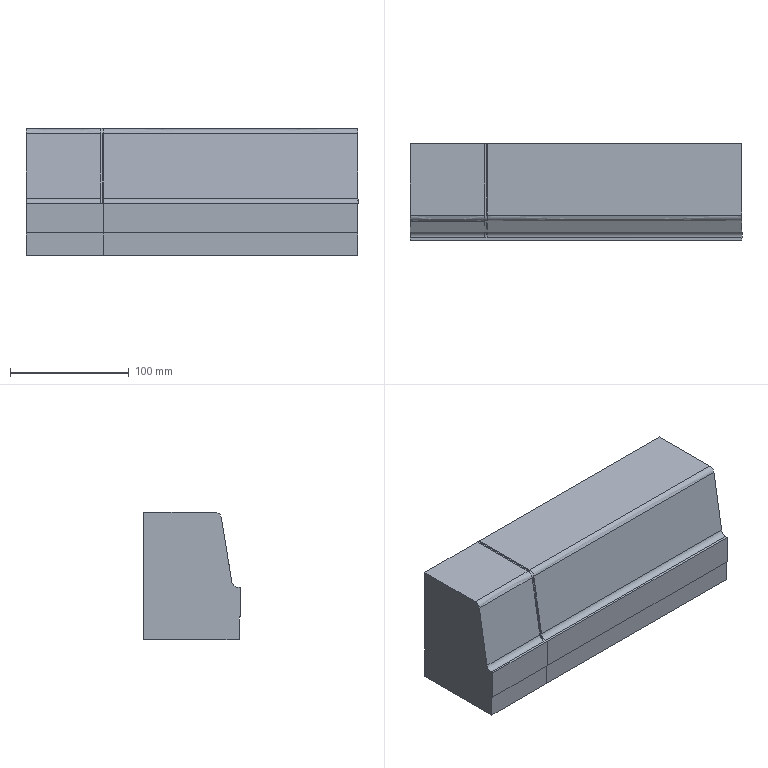Part | NX | features solid 2 | 1 solid | 36 faces | box 280 x 81.346 x 107.138 mm | volume 2196752 mm3 | spline 13 | plane 10 | cylinder 9 | cone 3 | sphere 1 | commonest cylinder face diameters 10 x3 12 x3 20 x2 14 x1